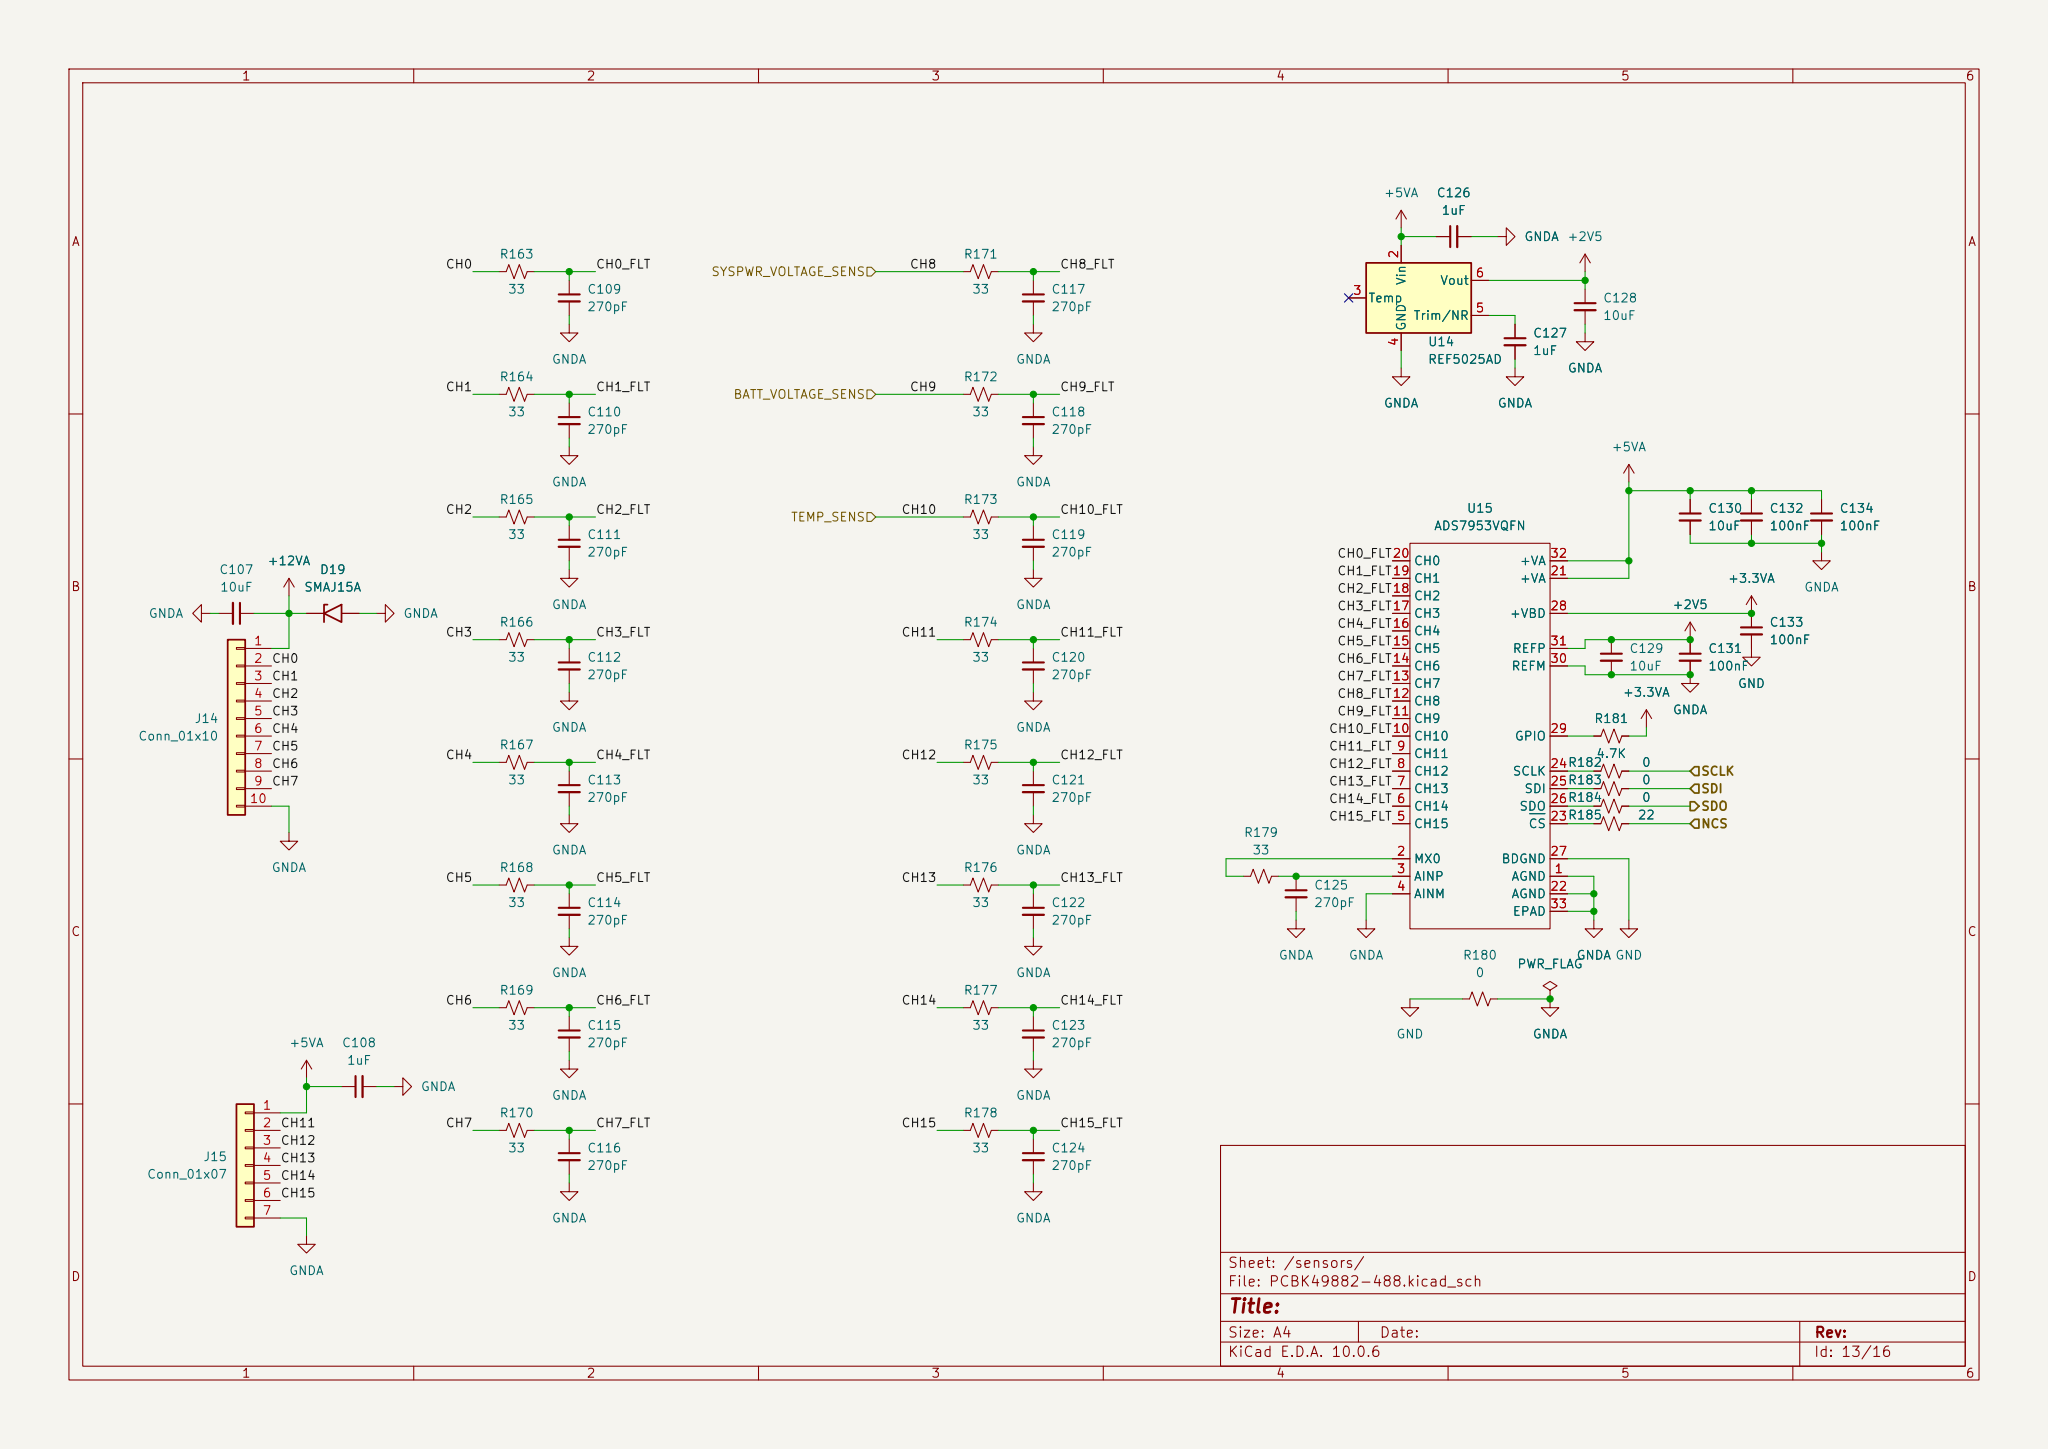Circuit board | KiCad | 536 parts | 438 nets | one sheet of the schematic
Parts on this sheet (reference | value | footprint):
C107 | 10uF | Capacitor_SMD:C_1210_3225Metric
C108 | 1uF | Capacitor_SMD:C_0603_1608Metric
C109
C110
C111
C112
C114
C115
C116
C117
C118
C119
C121
C123
C125
C126 | 1uF | Capacitor_SMD:C_0603_1608Metric
C127 | 1uF | Capacitor_SMD:C_0603_1608Metric
C128
C129
C130
C131
C132
C133
C134
D19 | SMAJ15A | Diode_SMD:D_SMA
J14 | Conn_01x10 | Connector_Molex:Molex_MicroClasp_55932-1030_1x10_P2.00mm_Vertical
J15 | Conn_01x07 | Connector_Molex:Molex_MicroClasp_55932-0730_1x07_P2.00mm_Vertical
R163
R164
R165
R166
R167
R168
R169
R170
R171
R172
R173
R174
R175
R176
R177
R178
R179
R180 | 0 | Resistor_SMD:R_0603_1608Metric
R181 | 4.7K | Resistor_SMD:R_0603_1608Metric
R182
R183
R184
R185 | 22 | Resistor_SMD:R_0603_1608Metric
U14 | REF5025AD | Package_SO:SOIC-8_3.9x4.9mm_P1.27mm
U15 | ADS7953VQFN | Package_User:VQFN-32_EP_5x5mm_Pitch0.5mm
Nets of these parts (net: part-pin ...):
+2V5: C128-1 C129-1 C131-1 U14-6 U15-31
+3.3VA: C133-1 R181-2 U15-28
+5VA: C108-1 C126-1 C130-1 C132-1 C134-1 J15-1 U14-2 U15-21 U15-32
+12VA: C107-1 D19-1 J14-1
/core_board_b2b/PB12{slash}SPI2_NCS: R185-2
/core_board_b2b/PB13{slash}SPI2_SCK: R182-2
/core_board_b2b/PB14{slash}SPI2_MISO: R183-2
/core_board_b2b/PB15{slash}SPI2_MOSI: R184-2
/sensors/CH0: J14-2 R163-1
/sensors/CH0_FLT: C109-1 R163-2 U15-20
/sensors/CH1: J14-3 R164-1
/sensors/CH1_FLT: C110-1 R164-2 U15-19
/sensors/CH2: J14-4 R165-1
/sensors/CH2_FLT: C111-1 R165-2 U15-18
/sensors/CH3: J14-5 R166-1
/sensors/CH3_FLT: C112-1 R166-2 U15-17
/sensors/CH4: J14-6 R167-1
/sensors/CH4_FLT: R167-2 U15-16
/sensors/CH5: J14-7 R168-1
/sensors/CH5_FLT: C114-1 R168-2 U15-15
/sensors/CH6: J14-8 R169-1
/sensors/CH6_FLT: C115-1 R169-2 U15-14
/sensors/CH7: J14-9 R170-1
/sensors/CH7_FLT: C116-1 R170-2 U15-13
/sensors/CH8: R171-1
/sensors/CH8_FLT: C117-1 R171-2 U15-12
/sensors/CH9: R172-1
/sensors/CH9_FLT: C118-1 R172-2 U15-11
/sensors/CH10: R173-1
/sensors/CH10_FLT: C119-1 R173-2 U15-10
/sensors/CH11: J15-2 R174-1
/sensors/CH11_FLT: R174-2 U15-9
/sensors/CH12: J15-3 R175-1
/sensors/CH12_FLT: C121-1 R175-2 U15-8
/sensors/CH13: J15-4 R176-1
/sensors/CH13_FLT: R176-2 U15-7
/sensors/CH14: J15-5 R177-1
/sensors/CH14_FLT: C123-1 R177-2 U15-6
/sensors/CH15: J15-6 R178-1
/sensors/CH15_FLT: R178-2 U15-5
GND: C133-2 R180-1 U15-27
GNDA: C107-2 C108-2 C109-2 C110-2 C111-2 C112-2 C114-2 C115-2 C116-2 C117-2 C118-2 C119-2 C121-2 C123-2 C125-2 C126-2 C127-2 C128-2 C129-2 C130-2 C131-2 C132-2 C134-2 D19-2 J14-10 J15-7 R180-2 U14-4 U15-1 U15-4 U15-22 U15-30 U15-33
Net-(U14-Trim{slash}NR): C127-1 U14-5
Net-(U15-AINP): C125-1 R179-2 U15-3
Net-(U15-GPIO): R181-1 U15-29
Net-(U15-MX0): R179-1 U15-2
Net-(U15-SCLK): R182-1 U15-24
Net-(U15-SDI): R183-1 U15-25
Net-(U15-SDO): R184-1 U15-26
Net-(U15-~{CS}): R185-1 U15-23
unconnected-(U14-DNC-Pad1): U14-1
unconnected-(U14-DNC-Pad8): U14-8
unconnected-(U14-NC-Pad7): U14-7
unconnected-(U14-Temp-Pad3): U14-3